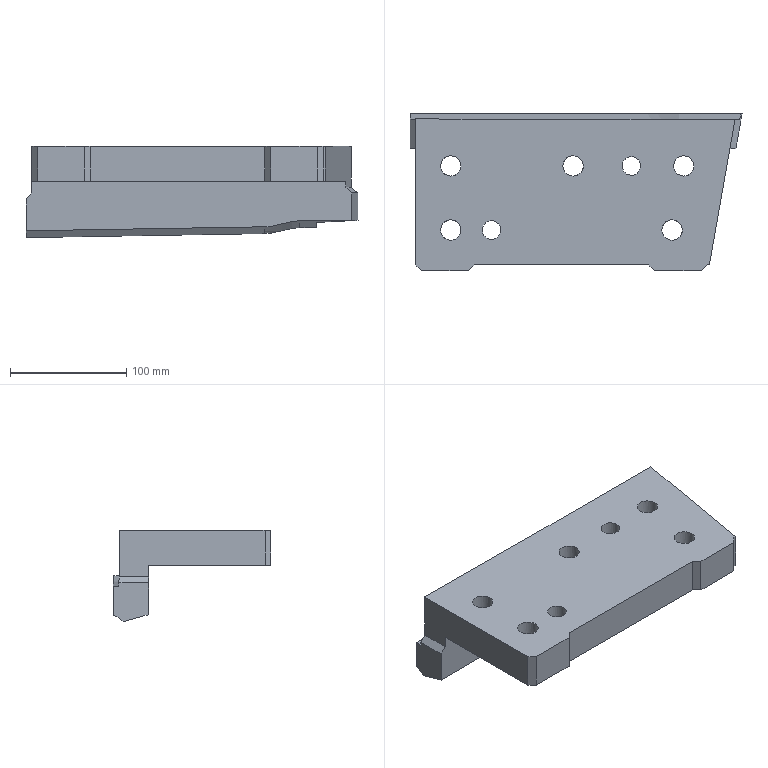Part | NX | features solid 2 | 1 solid | 48 faces | box 285.001 x 135.351 x 78.295 mm | volume 1268436 mm3 | plane 25 | cylinder 12 | spline 11 | commonest cylinder face diameters 17.5 x5 25 x5 16 x2